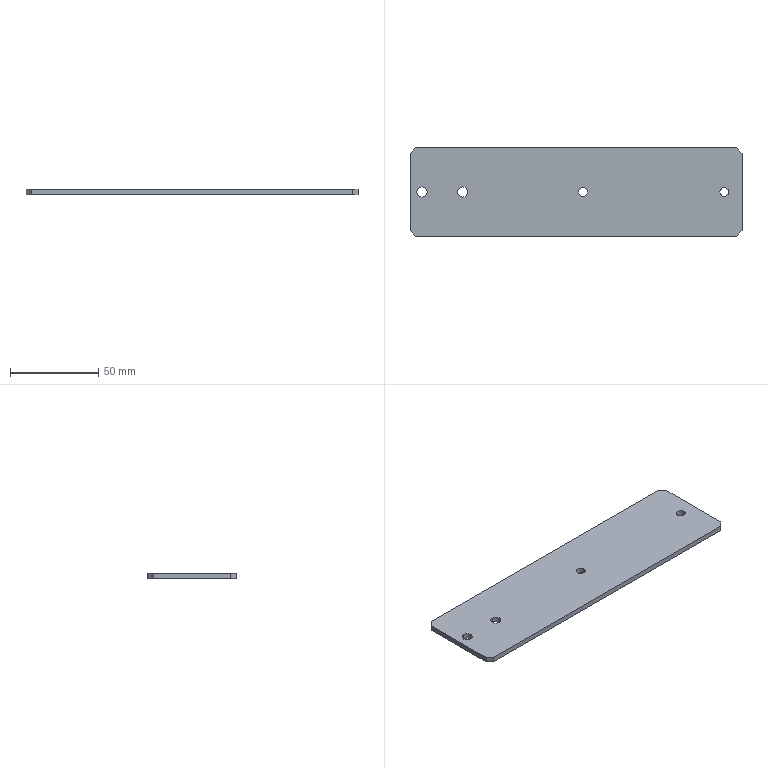Part | STEP file | J014-EBZ05-03-06-Part-1 | 1 solid | 18 faces | box 188 x 50 x 3 mm | volume 27870 mm3 | plane 10 | cylinder 8 | commonest cylinder face diameters 5 x4 5.8 x4
STEP:
#1=CARTESIAN_POINT('',(29.808,22.1,0.));
#2=VERTEX_POINT('',#1);
#3=CARTESIAN_POINT('',(29.808,27.9,0.));
#4=VERTEX_POINT('',#3);
#5=CARTESIAN_POINT('',(29.808,25.,0.));
#6=DIRECTION('',(0.,0.,-1.));
#7=DIRECTION('',(0.,1.,0.));
#8=AXIS2_PLACEMENT_3D('',#5,#6,#7);
#9=CIRCLE('',#8,2.9);
#10=EDGE_CURVE('',#2,#4,#9,.T.);
#11=ORIENTED_EDGE('',*,*,#10,.T.);
#12=CARTESIAN_POINT('',(29.808,27.9,3.));
#13=VERTEX_POINT('',#12);
#14=CARTESIAN_POINT('',(29.808,27.9,-1.8));
#15=DIRECTION('',(0.,0.,1.));
#16=VECTOR('',#15,1000.);
#17=LINE('',#14,#16);
#18=EDGE_CURVE('',#4,#13,#17,.T.);
#19=ORIENTED_EDGE('',*,*,#18,.T.);
#20=CARTESIAN_POINT('',(29.808,22.1,3.));
#21=VERTEX_POINT('',#20);
#22=CARTESIAN_POINT('',(29.808,25.,3.));
#23=DIRECTION('',(0.,0.,1.));
#24=DIRECTION('',(0.,-1.,0.));
#25=AXIS2_PLACEMENT_3D('',#22,#23,#24);
#26=CIRCLE('',#25,2.9);
#27=EDGE_CURVE('',#13,#21,#26,.T.);
#28=ORIENTED_EDGE('',*,*,#27,.T.);
#29=CARTESIAN_POINT('',(29.808,22.1,-1.8));
#30=DIRECTION('',(0.,0.,1.));
#31=VECTOR('',#30,1000.);
#32=LINE('',#29,#31);
#33=EDGE_CURVE('',#2,#21,#32,.T.);
#34=ORIENTED_EDGE('',*,*,#33,.F.);
#35=EDGE_LOOP('',(#11,#19,#28,#34));
#36=FACE_OUTER_BOUND('',#35,.T.);
#37=CARTESIAN_POINT('',(29.808,25.,-1.8));
#38=DIRECTION('',(0.,0.,1.));
#39=DIRECTION('',(0.,-1.,0.));
#40=AXIS2_PLACEMENT_3D('',#37,#38,#39);
#41=CYLINDRICAL_SURFACE('',#40,2.9);
#42=ADVANCED_FACE('',(#36),#41,.F.);
#43=CARTESIAN_POINT('',(6.808,22.1,0.));
#44=VERTEX_POINT('',#43);
#45=CARTESIAN_POINT('',(6.808,27.9,0.));
#46=VERTEX_POINT('',#45);
#47=CARTESIAN_POINT('',(6.808,25.,0.));
#48=DIRECTION('',(0.,0.,-1.));
#49=DIRECTION('',(0.,1.,0.));
#50=AXIS2_PLACEMENT_3D('',#47,#48,#49);
#51=CIRCLE('',#50,2.9);
#52=EDGE_CURVE('',#44,#46,#51,.T.);
#53=ORIENTED_EDGE('',*,*,#52,.T.);
#54=CARTESIAN_POINT('',(6.808,27.9,3.));
#55=VERTEX_POINT('',#54);
#56=CARTESIAN_POINT('',(6.808,27.9,-1.8));
#57=DIRECTION('',(0.,0.,1.));
#58=VECTOR('',#57,1000.);
#59=LINE('',#56,#58);
#60=EDGE_CURVE('',#46,#55,#59,.T.);
#61=ORIENTED_EDGE('',*,*,#60,.T.);
#62=CARTESIAN_POINT('',(6.808,22.1,3.));
#63=VERTEX_POINT('',#62);
#64=CARTESIAN_POINT('',(6.808,25.,3.));
#65=DIRECTION('',(0.,0.,1.));
#66=DIRECTION('',(0.,-1.,0.));
#67=AXIS2_PLACEMENT_3D('',#64,#65,#66);
#68=CIRCLE('',#67,2.9);
#69=EDGE_CURVE('',#55,#63,#68,.T.);
#70=ORIENTED_EDGE('',*,*,#69,.T.);
#71=CARTESIAN_POINT('',(6.808,22.1,-1.8));
#72=DIRECTION('',(0.,0.,1.));
#73=VECTOR('',#72,1000.);
#74=LINE('',#71,#73);
#75=EDGE_CURVE('',#44,#63,#74,.T.);
#76=ORIENTED_EDGE('',*,*,#75,.F.);
#77=EDGE_LOOP('',(#53,#61,#70,#76));
#78=FACE_OUTER_BOUND('',#77,.T.);
#79=CARTESIAN_POINT('',(6.808,25.,-1.8));
#80=DIRECTION('',(0.,0.,1.));
#81=DIRECTION('',(0.,-1.,0.));
#82=AXIS2_PLACEMENT_3D('',#79,#80,#81);
#83=CYLINDRICAL_SURFACE('',#82,2.9);
#84=ADVANCED_FACE('',(#78),#83,.F.);
#85=CARTESIAN_POINT('',(180.5,25.,0.));
#86=VERTEX_POINT('',#85);
#87=CARTESIAN_POINT('',(175.5,25.,0.));
#88=VERTEX_POINT('',#87);
#89=CARTESIAN_POINT('',(178.,25.,0.));
#90=DIRECTION('',(0.,0.,1.));
#91=DIRECTION('',(-1.,0.,0.));
#92=AXIS2_PLACEMENT_3D('',#89,#90,#91);
#93=CIRCLE('',#92,2.5);
#94=EDGE_CURVE('',#86,#88,#93,.T.);
#95=ORIENTED_EDGE('',*,*,#94,.F.);
#96=CARTESIAN_POINT('',(180.5,25.,3.));
#97=VERTEX_POINT('',#96);
#98=CARTESIAN_POINT('',(180.5,25.,0.));
#99=DIRECTION('',(0.,0.,1.));
#100=VECTOR('',#99,1000.);
#101=LINE('',#98,#100);
#102=EDGE_CURVE('',#86,#97,#101,.T.);
#103=ORIENTED_EDGE('',*,*,#102,.T.);
#104=CARTESIAN_POINT('',(175.5,25.,3.));
#105=VERTEX_POINT('',#104);
#106=CARTESIAN_POINT('',(178.,25.,3.));
#107=DIRECTION('',(0.,0.,-1.));
#108=DIRECTION('',(1.,0.,0.));
#109=AXIS2_PLACEMENT_3D('',#106,#107,#108);
#110=CIRCLE('',#109,2.5);
#111=EDGE_CURVE('',#105,#97,#110,.T.);
#112=ORIENTED_EDGE('',*,*,#111,.F.);
#113=CARTESIAN_POINT('',(175.5,25.,0.));
#114=DIRECTION('',(0.,0.,1.));
#115=VECTOR('',#114,1000.);
#116=LINE('',#113,#115);
#117=EDGE_CURVE('',#88,#105,#116,.T.);
#118=ORIENTED_EDGE('',*,*,#117,.F.);
#119=EDGE_LOOP('',(#95,#103,#112,#118));
#120=FACE_OUTER_BOUND('',#119,.T.);
#121=CARTESIAN_POINT('',(178.,25.,0.));
#122=DIRECTION('',(0.,0.,1.));
#123=DIRECTION('',(-1.,0.,0.));
#124=AXIS2_PLACEMENT_3D('',#121,#122,#123);
#125=CYLINDRICAL_SURFACE('',#124,2.5);
#126=ADVANCED_FACE('',(#120),#125,.F.);
#127=CARTESIAN_POINT('',(100.5,25.,0.));
#128=VERTEX_POINT('',#127);
#129=CARTESIAN_POINT('',(95.5,25.,0.));
#130=VERTEX_POINT('',#129);
#131=CARTESIAN_POINT('',(98.,25.,0.));
#132=DIRECTION('',(0.,0.,1.));
#133=DIRECTION('',(-1.,0.,0.));
#134=AXIS2_PLACEMENT_3D('',#131,#132,#133);
#135=CIRCLE('',#134,2.5);
#136=EDGE_CURVE('',#128,#130,#135,.T.);
#137=ORIENTED_EDGE('',*,*,#136,.F.);
#138=CARTESIAN_POINT('',(100.5,25.,3.));
#139=VERTEX_POINT('',#138);
#140=CARTESIAN_POINT('',(100.5,25.,0.));
#141=DIRECTION('',(0.,0.,1.));
#142=VECTOR('',#141,1000.);
#143=LINE('',#140,#142);
#144=EDGE_CURVE('',#128,#139,#143,.T.);
#145=ORIENTED_EDGE('',*,*,#144,.T.);
#146=CARTESIAN_POINT('',(95.5,25.,3.));
#147=VERTEX_POINT('',#146);
#148=CARTESIAN_POINT('',(98.,25.,3.));
#149=DIRECTION('',(0.,0.,-1.));
#150=DIRECTION('',(1.,0.,0.));
#151=AXIS2_PLACEMENT_3D('',#148,#149,#150);
#152=CIRCLE('',#151,2.5);
#153=EDGE_CURVE('',#147,#139,#152,.T.);
#154=ORIENTED_EDGE('',*,*,#153,.F.);
#155=CARTESIAN_POINT('',(95.5,25.,0.));
#156=DIRECTION('',(0.,0.,1.));
#157=VECTOR('',#156,1000.);
#158=LINE('',#155,#157);
#159=EDGE_CURVE('',#130,#147,#158,.T.);
#160=ORIENTED_EDGE('',*,*,#159,.F.);
#161=EDGE_LOOP('',(#137,#145,#154,#160));
#162=FACE_OUTER_BOUND('',#161,.T.);
#163=CARTESIAN_POINT('',(98.,25.,0.));
#164=DIRECTION('',(0.,0.,1.));
#165=DIRECTION('',(-1.,0.,0.));
#166=AXIS2_PLACEMENT_3D('',#163,#164,#165);
#167=CYLINDRICAL_SURFACE('',#166,2.5);
#168=ADVANCED_FACE('',(#162),#167,.F.);
#169=CARTESIAN_POINT('',(185.,0.,0.));
#170=VERTEX_POINT('',#169);
#171=CARTESIAN_POINT('',(3.,0.,0.));
#172=VERTEX_POINT('',#171);
#173=CARTESIAN_POINT('',(94.,0.,0.));
#174=DIRECTION('',(-1.,0.,0.));
#175=VECTOR('',#174,1000.);
#176=LINE('',#173,#175);
#177=EDGE_CURVE('',#170,#172,#176,.T.);
#178=ORIENTED_EDGE('',*,*,#177,.F.);
#179=CARTESIAN_POINT('',(185.,0.,3.));
#180=VERTEX_POINT('',#179);
#181=CARTESIAN_POINT('',(185.,0.,1.5));
#182=DIRECTION('',(0.,0.,1.));
#183=VECTOR('',#182,1000.);
#184=LINE('',#181,#183);
#185=EDGE_CURVE('',#170,#180,#184,.T.);
#186=ORIENTED_EDGE('',*,*,#185,.T.);
#187=CARTESIAN_POINT('',(3.,0.,3.));
#188=VERTEX_POINT('',#187);
#189=CARTESIAN_POINT('',(94.,0.,3.));
#190=DIRECTION('',(1.,0.,0.));
#191=VECTOR('',#190,1000.);
#192=LINE('',#189,#191);
#193=EDGE_CURVE('',#188,#180,#192,.T.);
#194=ORIENTED_EDGE('',*,*,#193,.F.);
#195=CARTESIAN_POINT('',(3.,0.,1.5));
#196=DIRECTION('',(0.,0.,-1.));
#197=VECTOR('',#196,1000.);
#198=LINE('',#195,#197);
#199=EDGE_CURVE('',#188,#172,#198,.T.);
#200=ORIENTED_EDGE('',*,*,#199,.T.);
#201=EDGE_LOOP('',(#178,#186,#194,#200));
#202=FACE_OUTER_BOUND('',#201,.T.);
#203=CARTESIAN_POINT('',(94.,0.,1.5));
#204=DIRECTION('',(0.,-1.,0.));
#205=DIRECTION('',(1.,0.,0.));
#206=AXIS2_PLACEMENT_3D('',#203,#204,#205);
#207=PLANE('',#206);
#208=ADVANCED_FACE('',(#202),#207,.T.);
#209=ORIENTED_EDGE('',*,*,#10,.F.);
#210=CARTESIAN_POINT('',(29.808,25.,0.));
#211=DIRECTION('',(0.,0.,-1.));
#212=DIRECTION('',(0.,1.,0.));
#213=AXIS2_PLACEMENT_3D('',#210,#211,#212);
#214=CIRCLE('',#213,2.9);
#215=EDGE_CURVE('',#4,#2,#214,.T.);
#216=ORIENTED_EDGE('',*,*,#215,.F.);
#217=EDGE_LOOP('',(#209,#216));
#218=FACE_BOUND('',#217,.T.);
#219=ORIENTED_EDGE('',*,*,#52,.F.);
#220=CARTESIAN_POINT('',(6.808,25.,0.));
#221=DIRECTION('',(0.,0.,-1.));
#222=DIRECTION('',(0.,1.,0.));
#223=AXIS2_PLACEMENT_3D('',#220,#221,#222);
#224=CIRCLE('',#223,2.9);
#225=EDGE_CURVE('',#46,#44,#224,.T.);
#226=ORIENTED_EDGE('',*,*,#225,.F.);
#227=EDGE_LOOP('',(#219,#226));
#228=FACE_BOUND('',#227,.T.);
#229=CARTESIAN_POINT('',(178.,25.,0.));
#230=DIRECTION('',(0.,0.,1.));
#231=DIRECTION('',(-1.,0.,0.));
#232=AXIS2_PLACEMENT_3D('',#229,#230,#231);
#233=CIRCLE('',#232,2.5);
#234=EDGE_CURVE('',#88,#86,#233,.T.);
#235=ORIENTED_EDGE('',*,*,#234,.T.);
#236=ORIENTED_EDGE('',*,*,#94,.T.);
#237=EDGE_LOOP('',(#235,#236));
#238=FACE_BOUND('',#237,.T.);
#239=CARTESIAN_POINT('',(98.,25.,0.));
#240=DIRECTION('',(0.,0.,1.));
#241=DIRECTION('',(-1.,0.,0.));
#242=AXIS2_PLACEMENT_3D('',#239,#240,#241);
#243=CIRCLE('',#242,2.5);
#244=EDGE_CURVE('',#130,#128,#243,.T.);
#245=ORIENTED_EDGE('',*,*,#244,.T.);
#246=ORIENTED_EDGE('',*,*,#136,.T.);
#247=EDGE_LOOP('',(#245,#246));
#248=FACE_BOUND('',#247,.T.);
#249=CARTESIAN_POINT('',(3.,50.,0.));
#250=VERTEX_POINT('',#249);
#251=CARTESIAN_POINT('',(185.,50.,0.));
#252=VERTEX_POINT('',#251);
#253=CARTESIAN_POINT('',(94.,50.,0.));
#254=DIRECTION('',(1.,0.,0.));
#255=VECTOR('',#254,1000.);
#256=LINE('',#253,#255);
#257=EDGE_CURVE('',#250,#252,#256,.T.);
#258=ORIENTED_EDGE('',*,*,#257,.T.);
#259=CARTESIAN_POINT('',(188.,47.,0.));
#260=VERTEX_POINT('',#259);
#261=CARTESIAN_POINT('',(139.5,95.5,0.));
#262=DIRECTION('',(0.7071,-0.7071,0.));
#263=VECTOR('',#262,1000.);
#264=LINE('',#261,#263);
#265=EDGE_CURVE('',#252,#260,#264,.T.);
#266=ORIENTED_EDGE('',*,*,#265,.T.);
#267=CARTESIAN_POINT('',(188.,3.,0.));
#268=VERTEX_POINT('',#267);
#269=CARTESIAN_POINT('',(188.,50.,0.));
#270=DIRECTION('',(0.,-1.,0.));
#271=VECTOR('',#270,1000.);
#272=LINE('',#269,#271);
#273=EDGE_CURVE('',#260,#268,#272,.T.);
#274=ORIENTED_EDGE('',*,*,#273,.T.);
#275=CARTESIAN_POINT('',(164.5,-20.5,0.));
#276=DIRECTION('',(-0.7071,-0.7071,0.));
#277=VECTOR('',#276,1000.);
#278=LINE('',#275,#277);
#279=EDGE_CURVE('',#268,#170,#278,.T.);
#280=ORIENTED_EDGE('',*,*,#279,.T.);
#281=ORIENTED_EDGE('',*,*,#177,.T.);
#282=CARTESIAN_POINT('',(0.,3.,0.));
#283=VERTEX_POINT('',#282);
#284=CARTESIAN_POINT('',(23.5,-20.5,0.));
#285=DIRECTION('',(-0.7071,0.7071,0.));
#286=VECTOR('',#285,1000.);
#287=LINE('',#284,#286);
#288=EDGE_CURVE('',#172,#283,#287,.T.);
#289=ORIENTED_EDGE('',*,*,#288,.T.);
#290=CARTESIAN_POINT('',(0.,47.,0.));
#291=VERTEX_POINT('',#290);
#292=CARTESIAN_POINT('',(0.,50.,0.));
#293=DIRECTION('',(0.,-1.,0.));
#294=VECTOR('',#293,1000.);
#295=LINE('',#292,#294);
#296=EDGE_CURVE('',#291,#283,#295,.T.);
#297=ORIENTED_EDGE('',*,*,#296,.F.);
#298=CARTESIAN_POINT('',(48.5,95.5,0.));
#299=DIRECTION('',(0.7071,0.7071,0.));
#300=VECTOR('',#299,1000.);
#301=LINE('',#298,#300);
#302=EDGE_CURVE('',#291,#250,#301,.T.);
#303=ORIENTED_EDGE('',*,*,#302,.T.);
#304=EDGE_LOOP('',(#258,#266,#274,#280,#281,#289,#297,#303));
#305=FACE_OUTER_BOUND('',#304,.T.);
#306=CARTESIAN_POINT('',(94.,50.,0.));
#307=DIRECTION('',(0.,0.,-1.));
#308=DIRECTION('',(0.,1.,0.));
#309=AXIS2_PLACEMENT_3D('',#306,#307,#308);
#310=PLANE('',#309);
#311=ADVANCED_FACE('',(#218,#228,#238,#248,#305),#310,.T.);
#312=ORIENTED_EDGE('',*,*,#296,.T.);
#313=CARTESIAN_POINT('',(0.,3.,3.));
#314=VERTEX_POINT('',#313);
#315=CARTESIAN_POINT('',(0.,3.,1.5));
#316=DIRECTION('',(0.,0.,1.));
#317=VECTOR('',#316,1000.);
#318=LINE('',#315,#317);
#319=EDGE_CURVE('',#283,#314,#318,.T.);
#320=ORIENTED_EDGE('',*,*,#319,.T.);
#321=CARTESIAN_POINT('',(0.,47.,3.));
#322=VERTEX_POINT('',#321);
#323=CARTESIAN_POINT('',(0.,50.,3.));
#324=DIRECTION('',(0.,-1.,0.));
#325=VECTOR('',#324,1000.);
#326=LINE('',#323,#325);
#327=EDGE_CURVE('',#322,#314,#326,.T.);
#328=ORIENTED_EDGE('',*,*,#327,.F.);
#329=CARTESIAN_POINT('',(0.,47.,1.5));
#330=DIRECTION('',(0.,0.,-1.));
#331=VECTOR('',#330,1000.);
#332=LINE('',#329,#331);
#333=EDGE_CURVE('',#322,#291,#332,.T.);
#334=ORIENTED_EDGE('',*,*,#333,.T.);
#335=EDGE_LOOP('',(#312,#320,#328,#334));
#336=FACE_OUTER_BOUND('',#335,.T.);
#337=CARTESIAN_POINT('',(0.,50.,1.5));
#338=DIRECTION('',(-1.,0.,0.));
#339=DIRECTION('',(0.,-1.,0.));
#340=AXIS2_PLACEMENT_3D('',#337,#338,#339);
#341=PLANE('',#340);
#342=ADVANCED_FACE('',(#336),#341,.T.);
#343=CARTESIAN_POINT('',(29.808,25.,3.));
#344=DIRECTION('',(0.,0.,1.));
#345=DIRECTION('',(0.,-1.,0.));
#346=AXIS2_PLACEMENT_3D('',#343,#344,#345);
#347=CIRCLE('',#346,2.9);
#348=EDGE_CURVE('',#21,#13,#347,.T.);
#349=ORIENTED_EDGE('',*,*,#348,.F.);
#350=ORIENTED_EDGE('',*,*,#27,.F.);
#351=EDGE_LOOP('',(#349,#350));
#352=FACE_BOUND('',#351,.T.);
#353=CARTESIAN_POINT('',(6.808,25.,3.));
#354=DIRECTION('',(0.,0.,1.));
#355=DIRECTION('',(0.,-1.,0.));
#356=AXIS2_PLACEMENT_3D('',#353,#354,#355);
#357=CIRCLE('',#356,2.9);
#358=EDGE_CURVE('',#63,#55,#357,.T.);
#359=ORIENTED_EDGE('',*,*,#358,.F.);
#360=ORIENTED_EDGE('',*,*,#69,.F.);
#361=EDGE_LOOP('',(#359,#360));
#362=FACE_BOUND('',#361,.T.);
#363=ORIENTED_EDGE('',*,*,#111,.T.);
#364=CARTESIAN_POINT('',(178.,25.,3.));
#365=DIRECTION('',(0.,0.,-1.));
#366=DIRECTION('',(1.,0.,0.));
#367=AXIS2_PLACEMENT_3D('',#364,#365,#366);
#368=CIRCLE('',#367,2.5);
#369=EDGE_CURVE('',#97,#105,#368,.T.);
#370=ORIENTED_EDGE('',*,*,#369,.T.);
#371=EDGE_LOOP('',(#363,#370));
#372=FACE_BOUND('',#371,.T.);
#373=ORIENTED_EDGE('',*,*,#153,.T.);
#374=CARTESIAN_POINT('',(98.,25.,3.));
#375=DIRECTION('',(0.,0.,-1.));
#376=DIRECTION('',(1.,0.,0.));
#377=AXIS2_PLACEMENT_3D('',#374,#375,#376);
#378=CIRCLE('',#377,2.5);
#379=EDGE_CURVE('',#139,#147,#378,.T.);
#380=ORIENTED_EDGE('',*,*,#379,.T.);
#381=EDGE_LOOP('',(#373,#380));
#382=FACE_BOUND('',#381,.T.);
#383=CARTESIAN_POINT('',(188.,47.,3.));
#384=VERTEX_POINT('',#383);
#385=CARTESIAN_POINT('',(188.,3.,3.));
#386=VERTEX_POINT('',#385);
#387=CARTESIAN_POINT('',(188.,50.,3.));
#388=DIRECTION('',(0.,-1.,0.));
#389=VECTOR('',#388,1000.);
#390=LINE('',#387,#389);
#391=EDGE_CURVE('',#384,#386,#390,.T.);
#392=ORIENTED_EDGE('',*,*,#391,.F.);
#393=CARTESIAN_POINT('',(185.,50.,3.));
#394=VERTEX_POINT('',#393);
#395=CARTESIAN_POINT('',(139.5,95.5,3.));
#396=DIRECTION('',(-0.7071,0.7071,0.));
#397=VECTOR('',#396,1000.);
#398=LINE('',#395,#397);
#399=EDGE_CURVE('',#384,#394,#398,.T.);
#400=ORIENTED_EDGE('',*,*,#399,.T.);
#401=CARTESIAN_POINT('',(3.,50.,3.));
#402=VERTEX_POINT('',#401);
#403=CARTESIAN_POINT('',(94.,50.,3.));
#404=DIRECTION('',(-1.,0.,0.));
#405=VECTOR('',#404,1000.);
#406=LINE('',#403,#405);
#407=EDGE_CURVE('',#394,#402,#406,.T.);
#408=ORIENTED_EDGE('',*,*,#407,.T.);
#409=CARTESIAN_POINT('',(48.5,95.5,3.));
#410=DIRECTION('',(-0.7071,-0.7071,0.));
#411=VECTOR('',#410,1000.);
#412=LINE('',#409,#411);
#413=EDGE_CURVE('',#402,#322,#412,.T.);
#414=ORIENTED_EDGE('',*,*,#413,.T.);
#415=ORIENTED_EDGE('',*,*,#327,.T.);
#416=CARTESIAN_POINT('',(23.5,-20.5,3.));
#417=DIRECTION('',(0.7071,-0.7071,0.));
#418=VECTOR('',#417,1000.);
#419=LINE('',#416,#418);
#420=EDGE_CURVE('',#314,#188,#419,.T.);
#421=ORIENTED_EDGE('',*,*,#420,.T.);
#422=ORIENTED_EDGE('',*,*,#193,.T.);
#423=CARTESIAN_POINT('',(164.5,-20.5,3.));
#424=DIRECTION('',(0.7071,0.7071,0.));
#425=VECTOR('',#424,1000.);
#426=LINE('',#423,#425);
#427=EDGE_CURVE('',#180,#386,#426,.T.);
#428=ORIENTED_EDGE('',*,*,#427,.T.);
#429=EDGE_LOOP('',(#392,#400,#408,#414,#415,#421,#422,#428));
#430=FACE_OUTER_BOUND('',#429,.T.);
#431=CARTESIAN_POINT('',(94.,50.,3.));
#432=DIRECTION('',(0.,0.,1.));
#433=DIRECTION('',(0.,-1.,0.));
#434=AXIS2_PLACEMENT_3D('',#431,#432,#433);
#435=PLANE('',#434);
#436=ADVANCED_FACE('',(#352,#362,#372,#382,#430),#435,.T.);
#437=ORIENTED_EDGE('',*,*,#407,.F.);
#438=CARTESIAN_POINT('',(185.,50.,1.5));
#439=DIRECTION('',(0.,0.,-1.));
#440=VECTOR('',#439,1000.);
#441=LINE('',#438,#440);
#442=EDGE_CURVE('',#394,#252,#441,.T.);
#443=ORIENTED_EDGE('',*,*,#442,.T.);
#444=ORIENTED_EDGE('',*,*,#257,.F.);
#445=CARTESIAN_POINT('',(3.,50.,1.5));
#446=DIRECTION('',(0.,0.,1.));
#447=VECTOR('',#446,1000.);
#448=LINE('',#445,#447);
#449=EDGE_CURVE('',#250,#402,#448,.T.);
#450=ORIENTED_EDGE('',*,*,#449,.T.);
#451=EDGE_LOOP('',(#437,#443,#444,#450));
#452=FACE_OUTER_BOUND('',#451,.T.);
#453=CARTESIAN_POINT('',(94.,50.,1.5));
#454=DIRECTION('',(0.,1.,0.));
#455=DIRECTION('',(-1.,0.,0.));
#456=AXIS2_PLACEMENT_3D('',#453,#454,#455);
#457=PLANE('',#456);
#458=ADVANCED_FACE('',(#452),#457,.T.);
#459=ORIENTED_EDGE('',*,*,#273,.F.);
#460=CARTESIAN_POINT('',(188.,47.,1.5));
#461=DIRECTION('',(0.,0.,1.));
#462=VECTOR('',#461,1000.);
#463=LINE('',#460,#462);
#464=EDGE_CURVE('',#260,#384,#463,.T.);
#465=ORIENTED_EDGE('',*,*,#464,.T.);
#466=ORIENTED_EDGE('',*,*,#391,.T.);
#467=CARTESIAN_POINT('',(188.,3.,1.5));
#468=DIRECTION('',(0.,0.,-1.));
#469=VECTOR('',#468,1000.);
#470=LINE('',#467,#469);
#471=EDGE_CURVE('',#386,#268,#470,.T.);
#472=ORIENTED_EDGE('',*,*,#471,.T.);
#473=EDGE_LOOP('',(#459,#465,#466,#472));
#474=FACE_OUTER_BOUND('',#473,.T.);
#475=CARTESIAN_POINT('',(188.,50.,1.5));
#476=DIRECTION('',(1.,0.,0.));
#477=DIRECTION('',(0.,1.,0.));
#478=AXIS2_PLACEMENT_3D('',#475,#476,#477);
#479=PLANE('',#478);
#480=ADVANCED_FACE('',(#474),#479,.T.);
#481=ORIENTED_EDGE('',*,*,#144,.F.);
#482=ORIENTED_EDGE('',*,*,#244,.F.);
#483=ORIENTED_EDGE('',*,*,#159,.T.);
#484=ORIENTED_EDGE('',*,*,#379,.F.);
#485=EDGE_LOOP('',(#481,#482,#483,#484));
#486=FACE_OUTER_BOUND('',#485,.T.);
#487=CARTESIAN_POINT('',(98.,25.,0.));
#488=DIRECTION('',(0.,0.,1.));
#489=DIRECTION('',(-1.,0.,0.));
#490=AXIS2_PLACEMENT_3D('',#487,#488,#489);
#491=CYLINDRICAL_SURFACE('',#490,2.5);
#492=ADVANCED_FACE('',(#486),#491,.F.);
#493=ORIENTED_EDGE('',*,*,#102,.F.);
#494=ORIENTED_EDGE('',*,*,#234,.F.);
#495=ORIENTED_EDGE('',*,*,#117,.T.);
#496=ORIENTED_EDGE('',*,*,#369,.F.);
#497=EDGE_LOOP('',(#493,#494,#495,#496));
#498=FACE_OUTER_BOUND('',#497,.T.);
#499=CARTESIAN_POINT('',(178.,25.,0.));
#500=DIRECTION('',(0.,0.,1.));
#501=DIRECTION('',(-1.,0.,0.));
#502=AXIS2_PLACEMENT_3D('',#499,#500,#501);
#503=CYLINDRICAL_SURFACE('',#502,2.5);
#504=ADVANCED_FACE('',(#498),#503,.F.);
#505=ORIENTED_EDGE('',*,*,#265,.F.);
#506=ORIENTED_EDGE('',*,*,#442,.F.);
#507=ORIENTED_EDGE('',*,*,#399,.F.);
#508=ORIENTED_EDGE('',*,*,#464,.F.);
#509=EDGE_LOOP('',(#505,#506,#507,#508));
#510=FACE_OUTER_BOUND('',#509,.T.);
#511=CARTESIAN_POINT('',(188.,47.,1.5));
#512=DIRECTION('',(-0.7071,-0.7071,0.));
#513=DIRECTION('',(0.,0.,1.));
#514=AXIS2_PLACEMENT_3D('',#511,#512,#513);
#515=PLANE('',#514);
#516=ADVANCED_FACE('',(#510),#515,.F.);
#517=ORIENTED_EDGE('',*,*,#427,.F.);
#518=ORIENTED_EDGE('',*,*,#185,.F.);
#519=ORIENTED_EDGE('',*,*,#279,.F.);
#520=ORIENTED_EDGE('',*,*,#471,.F.);
#521=EDGE_LOOP('',(#517,#518,#519,#520));
#522=FACE_OUTER_BOUND('',#521,.T.);
#523=CARTESIAN_POINT('',(188.,3.,1.5));
#524=DIRECTION('',(-0.7071,0.7071,0.));
#525=DIRECTION('',(0.,0.,-1.));
#526=AXIS2_PLACEMENT_3D('',#523,#524,#525);
#527=PLANE('',#526);
#528=ADVANCED_FACE('',(#522),#527,.F.);
#529=ORIENTED_EDGE('',*,*,#288,.F.);
#530=ORIENTED_EDGE('',*,*,#199,.F.);
#531=ORIENTED_EDGE('',*,*,#420,.F.);
#532=ORIENTED_EDGE('',*,*,#319,.F.);
#533=EDGE_LOOP('',(#529,#530,#531,#532));
#534=FACE_OUTER_BOUND('',#533,.T.);
#535=CARTESIAN_POINT('',(0.,3.,1.5));
#536=DIRECTION('',(0.7071,0.7071,0.));
#537=DIRECTION('',(0.,0.,1.));
#538=AXIS2_PLACEMENT_3D('',#535,#536,#537);
#539=PLANE('',#538);
#540=ADVANCED_FACE('',(#534),#539,.F.);
#541=ORIENTED_EDGE('',*,*,#413,.F.);
#542=ORIENTED_EDGE('',*,*,#449,.F.);
#543=ORIENTED_EDGE('',*,*,#302,.F.);
#544=ORIENTED_EDGE('',*,*,#333,.F.);
#545=EDGE_LOOP('',(#541,#542,#543,#544));
#546=FACE_OUTER_BOUND('',#545,.T.);
#547=CARTESIAN_POINT('',(0.,47.,1.5));
#548=DIRECTION('',(0.7071,-0.7071,0.));
#549=DIRECTION('',(0.,0.,-1.));
#550=AXIS2_PLACEMENT_3D('',#547,#548,#549);
#551=PLANE('',#550);
#552=ADVANCED_FACE('',(#546),#551,.F.);
#553=ORIENTED_EDGE('',*,*,#60,.F.);
#554=ORIENTED_EDGE('',*,*,#225,.T.);
#555=ORIENTED_EDGE('',*,*,#75,.T.);
#556=ORIENTED_EDGE('',*,*,#358,.T.);
#557=EDGE_LOOP('',(#553,#554,#555,#556));
#558=FACE_OUTER_BOUND('',#557,.T.);
#559=CARTESIAN_POINT('',(6.808,25.,-1.8));
#560=DIRECTION('',(0.,0.,1.));
#561=DIRECTION('',(0.,-1.,0.));
#562=AXIS2_PLACEMENT_3D('',#559,#560,#561);
#563=CYLINDRICAL_SURFACE('',#562,2.9);
#564=ADVANCED_FACE('',(#558),#563,.F.);
#565=ORIENTED_EDGE('',*,*,#18,.F.);
#566=ORIENTED_EDGE('',*,*,#215,.T.);
#567=ORIENTED_EDGE('',*,*,#33,.T.);
#568=ORIENTED_EDGE('',*,*,#348,.T.);
#569=EDGE_LOOP('',(#565,#566,#567,#568));
#570=FACE_OUTER_BOUND('',#569,.T.);
#571=CARTESIAN_POINT('',(29.808,25.,-1.8));
#572=DIRECTION('',(0.,0.,1.));
#573=DIRECTION('',(0.,-1.,0.));
#574=AXIS2_PLACEMENT_3D('',#571,#572,#573);
#575=CYLINDRICAL_SURFACE('',#574,2.9);
#576=ADVANCED_FACE('',(#570),#575,.F.);
#577=CLOSED_SHELL('',(#42,#84,#126,#168,#208,#311,#342,#436,#458,#480,#492,#504,#516,#528,#540,#552,#564,#576));
#578=MANIFOLD_SOLID_BREP('',#577);
#579=CARTESIAN_POINT('',(0.,0.,0.));
#580=DIRECTION('',(0.,0.,1.));
#581=DIRECTION('',(1.,0.,0.));
#582=AXIS2_PLACEMENT_3D('',#579,#580,#581);
#583=(LENGTH_UNIT()NAMED_UNIT(*)SI_UNIT(.MILLI.,.METRE.));
#584=UNCERTAINTY_MEASURE_WITH_UNIT(LENGTH_MEASURE(0.00001),#583,'','');
#585=(NAMED_UNIT(*)PLANE_ANGLE_UNIT()SI_UNIT($,.RADIAN.));
#586=(NAMED_UNIT(*)SI_UNIT($,.STERADIAN.)SOLID_ANGLE_UNIT());
#587=(GEOMETRIC_REPRESENTATION_CONTEXT(3)GLOBAL_UNCERTAINTY_ASSIGNED_CONTEXT((#584))GLOBAL_UNIT_ASSIGNED_CONTEXT((#583,#585,#586))REPRESENTATION_CONTEXT('',''));
#588=ADVANCED_BREP_SHAPE_REPRESENTATION('',(#578,#582),#587);